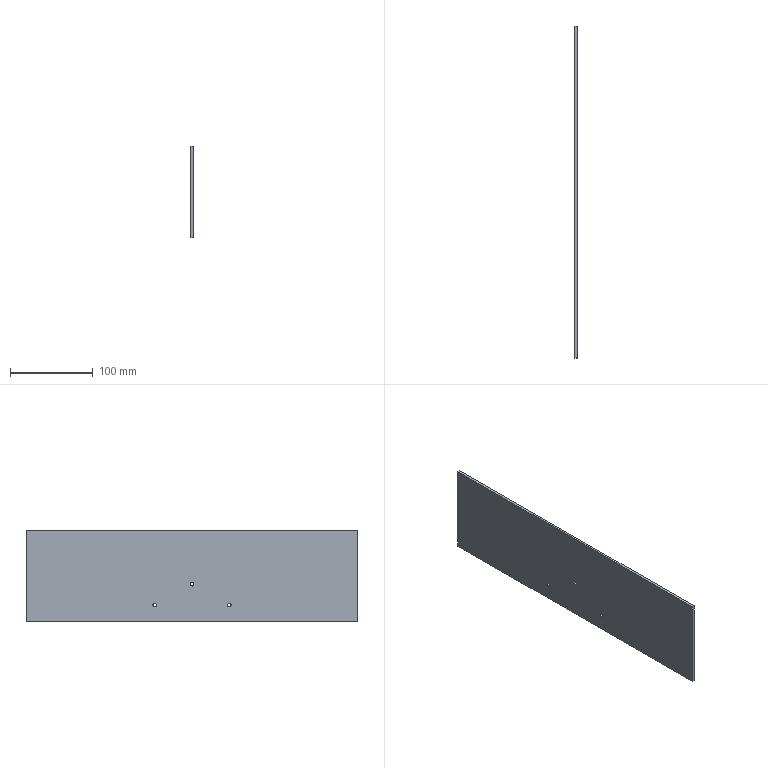Part | STEP file | HESS-408-70-15W-W-45-upper door right reinforcing plate | 1 solid | 12 faces | box 3 x 400 x 110 mm | volume 131875 mm3 | cylinder 6 | plane 6 | commonest cylinder face diameters 4.2 x6
STEP:
#1=CARTESIAN_POINT('',(0.,0.,0.));
#2=DIRECTION('',(0.,0.,1.));
#3=DIRECTION('',(1.,0.,0.));
#4=AXIS2_PLACEMENT_3D('',#1,#2,#3);
#5=CARTESIAN_POINT('',(-3.,-45.,-37.1));
#6=VERTEX_POINT('',#5);
#7=CARTESIAN_POINT('',(0.,-45.,-37.1));
#8=VERTEX_POINT('',#7);
#9=CARTESIAN_POINT('',(0.,-45.,-37.1));
#10=DIRECTION('',(1.,0.,0.));
#11=VECTOR('',#10,1.);
#12=LINE('',#9,#11);
#13=CARTESIAN_POINT('',(0.,-45.,-35.));
#14=DIRECTION('',(1.,0.,0.));
#15=DIRECTION('',(0.,0.,-1.));
#16=AXIS2_PLACEMENT_3D('',#13,#14,#15);
#17=CYLINDRICAL_SURFACE('',#16,2.1);
#18=CARTESIAN_POINT('',(6.283,0.));
#19=DIRECTION('',(0.,1.));
#20=VECTOR('',#19,1.);
#21=LINE('',#18,#20);
#22=(GEOMETRIC_REPRESENTATION_CONTEXT(2)PARAMETRIC_REPRESENTATION_CONTEXT()REPRESENTATION_CONTEXT('',''));
#23=DEFINITIONAL_REPRESENTATION('',(#21),#22);
#24=PCURVE('',#17,#23);
#25=CARTESIAN_POINT('',(0.,-45.,-35.));
#26=DIRECTION('',(1.,0.,0.));
#27=DIRECTION('',(0.,0.,-1.));
#28=AXIS2_PLACEMENT_3D('',#25,#26,#27);
#29=CYLINDRICAL_SURFACE('',#28,2.1);
#30=CARTESIAN_POINT('',(0.,0.));
#31=DIRECTION('',(0.,1.));
#32=VECTOR('',#31,1.);
#33=LINE('',#30,#32);
#34=(GEOMETRIC_REPRESENTATION_CONTEXT(2)PARAMETRIC_REPRESENTATION_CONTEXT()REPRESENTATION_CONTEXT('',''));
#35=DEFINITIONAL_REPRESENTATION('',(#33),#34);
#36=PCURVE('',#29,#35);
#37=SURFACE_CURVE('',#12,(#24,#36),.PCURVE_S1.);
#38=EDGE_CURVE('',#6,#8,#37,.T.);
#39=ORIENTED_EDGE('',*,*,#38,.T.);
#40=CARTESIAN_POINT('',(0.,-45.,-32.9));
#41=VERTEX_POINT('',#40);
#42=CARTESIAN_POINT('',(0.,-45.,-35.));
#43=DIRECTION('',(-1.,0.,0.));
#44=DIRECTION('',(0.,0.,-1.));
#45=AXIS2_PLACEMENT_3D('',#42,#43,#44);
#46=CIRCLE('',#45,2.1);
#47=CARTESIAN_POINT('',(6.283,0.));
#48=DIRECTION('',(-1.,0.));
#49=VECTOR('',#48,1.);
#50=LINE('',#47,#49);
#51=(GEOMETRIC_REPRESENTATION_CONTEXT(2)PARAMETRIC_REPRESENTATION_CONTEXT()REPRESENTATION_CONTEXT('',''));
#52=DEFINITIONAL_REPRESENTATION('',(#50),#51);
#53=PCURVE('',#17,#52);
#54=CARTESIAN_POINT('',(0.,0.,0.));
#55=DIRECTION('',(-1.,0.,0.));
#56=DIRECTION('',(0.,0.,1.));
#57=AXIS2_PLACEMENT_3D('',#54,#55,#56);
#58=PLANE('',#57);
#59=CARTESIAN_POINT('',(-35.,-45.));
#60=DIRECTION('',(-1.,0.));
#61=AXIS2_PLACEMENT_2D('',#59,#60);
#62=CIRCLE('',#61,2.1);
#63=(GEOMETRIC_REPRESENTATION_CONTEXT(2)PARAMETRIC_REPRESENTATION_CONTEXT()REPRESENTATION_CONTEXT('',''));
#64=DEFINITIONAL_REPRESENTATION('',(#62),#63);
#65=PCURVE('',#58,#64);
#66=SURFACE_CURVE('',#46,(#53,#65),.PCURVE_S1.);
#67=EDGE_CURVE('',#8,#41,#66,.T.);
#68=ORIENTED_EDGE('',*,*,#67,.T.);
#69=CARTESIAN_POINT('',(-3.,-45.,-32.9));
#70=VERTEX_POINT('',#69);
#71=CARTESIAN_POINT('',(0.,-45.,-32.9));
#72=DIRECTION('',(1.,0.,0.));
#73=VECTOR('',#72,1.);
#74=LINE('',#71,#73);
#75=CARTESIAN_POINT('',(3.142,0.));
#76=DIRECTION('',(0.,1.));
#77=VECTOR('',#76,1.);
#78=LINE('',#75,#77);
#79=(GEOMETRIC_REPRESENTATION_CONTEXT(2)PARAMETRIC_REPRESENTATION_CONTEXT()REPRESENTATION_CONTEXT('',''));
#80=DEFINITIONAL_REPRESENTATION('',(#78),#79);
#81=PCURVE('',#17,#80);
#82=CARTESIAN_POINT('',(3.142,0.));
#83=DIRECTION('',(0.,1.));
#84=VECTOR('',#83,1.);
#85=LINE('',#82,#84);
#86=(GEOMETRIC_REPRESENTATION_CONTEXT(2)PARAMETRIC_REPRESENTATION_CONTEXT()REPRESENTATION_CONTEXT('',''));
#87=DEFINITIONAL_REPRESENTATION('',(#85),#86);
#88=PCURVE('',#29,#87);
#89=SURFACE_CURVE('',#74,(#81,#88),.PCURVE_S1.);
#90=EDGE_CURVE('',#70,#41,#89,.T.);
#91=ORIENTED_EDGE('',*,*,#90,.F.);
#92=CARTESIAN_POINT('',(-3.,-45.,-35.));
#93=DIRECTION('',(1.,0.,0.));
#94=DIRECTION('',(0.,0.,-1.));
#95=AXIS2_PLACEMENT_3D('',#92,#93,#94);
#96=CIRCLE('',#95,2.1);
#97=CARTESIAN_POINT('',(0.,-3.));
#98=DIRECTION('',(1.,0.));
#99=VECTOR('',#98,1.);
#100=LINE('',#97,#99);
#101=(GEOMETRIC_REPRESENTATION_CONTEXT(2)PARAMETRIC_REPRESENTATION_CONTEXT()REPRESENTATION_CONTEXT('',''));
#102=DEFINITIONAL_REPRESENTATION('',(#100),#101);
#103=PCURVE('',#17,#102);
#104=CARTESIAN_POINT('',(-3.,0.,0.));
#105=DIRECTION('',(-1.,0.,0.));
#106=DIRECTION('',(0.,0.,1.));
#107=AXIS2_PLACEMENT_3D('',#104,#105,#106);
#108=PLANE('',#107);
#109=CARTESIAN_POINT('',(-37.1,-45.));
#110=CARTESIAN_POINT('',(-37.1,-41.363));
#111=CARTESIAN_POINT('',(-33.95,-43.181));
#112=CARTESIAN_POINT('',(-30.8,-45.));
#113=CARTESIAN_POINT('',(-33.95,-46.819));
#114=CARTESIAN_POINT('',(-37.1,-48.637));
#115=CARTESIAN_POINT('',(-37.1,-45.));
#116=(BOUNDED_CURVE()B_SPLINE_CURVE(2,(#109,#110,#111,#112,#113,#114,#115),.UNSPECIFIED.,.T.,.F.)B_SPLINE_CURVE_WITH_KNOTS((1,2,2,2,2,1),(-2.094,0.,2.094,4.189,6.283,8.378),.UNSPECIFIED.)CURVE()GEOMETRIC_REPRESENTATION_ITEM()RATIONAL_B_SPLINE_CURVE((1.,0.5,1.,0.5,1.,0.5,1.))REPRESENTATION_ITEM(''));
#117=(GEOMETRIC_REPRESENTATION_CONTEXT(2)PARAMETRIC_REPRESENTATION_CONTEXT()REPRESENTATION_CONTEXT('',''));
#118=DEFINITIONAL_REPRESENTATION('',(#116),#117);
#119=PCURVE('',#108,#118);
#120=SURFACE_CURVE('',#96,(#103,#119),.PCURVE_S1.);
#121=EDGE_CURVE('',#70,#6,#120,.T.);
#122=ORIENTED_EDGE('',*,*,#121,.T.);
#123=EDGE_LOOP('',(#39,#68,#91,#122));
#124=FACE_BOUND('',#123,.F.);
#125=ADVANCED_FACE('',(#124),#17,.F.);
#126=CARTESIAN_POINT('',(-3.,0.,-12.1));
#127=VERTEX_POINT('',#126);
#128=CARTESIAN_POINT('',(0.,0.,-12.1));
#129=VERTEX_POINT('',#128);
#130=CARTESIAN_POINT('',(0.,0.,-12.1));
#131=DIRECTION('',(1.,0.,0.));
#132=VECTOR('',#131,1.);
#133=LINE('',#130,#132);
#134=CARTESIAN_POINT('',(0.,0.,-10.));
#135=DIRECTION('',(1.,0.,0.));
#136=DIRECTION('',(0.,0.,-1.));
#137=AXIS2_PLACEMENT_3D('',#134,#135,#136);
#138=CYLINDRICAL_SURFACE('',#137,2.1);
#139=CARTESIAN_POINT('',(6.283,0.));
#140=DIRECTION('',(0.,1.));
#141=VECTOR('',#140,1.);
#142=LINE('',#139,#141);
#143=(GEOMETRIC_REPRESENTATION_CONTEXT(2)PARAMETRIC_REPRESENTATION_CONTEXT()REPRESENTATION_CONTEXT('',''));
#144=DEFINITIONAL_REPRESENTATION('',(#142),#143);
#145=PCURVE('',#138,#144);
#146=CARTESIAN_POINT('',(0.,0.,-10.));
#147=DIRECTION('',(1.,0.,0.));
#148=DIRECTION('',(0.,0.,-1.));
#149=AXIS2_PLACEMENT_3D('',#146,#147,#148);
#150=CYLINDRICAL_SURFACE('',#149,2.1);
#151=CARTESIAN_POINT('',(0.,0.));
#152=DIRECTION('',(0.,1.));
#153=VECTOR('',#152,1.);
#154=LINE('',#151,#153);
#155=(GEOMETRIC_REPRESENTATION_CONTEXT(2)PARAMETRIC_REPRESENTATION_CONTEXT()REPRESENTATION_CONTEXT('',''));
#156=DEFINITIONAL_REPRESENTATION('',(#154),#155);
#157=PCURVE('',#150,#156);
#158=SURFACE_CURVE('',#133,(#145,#157),.PCURVE_S1.);
#159=EDGE_CURVE('',#127,#129,#158,.T.);
#160=ORIENTED_EDGE('',*,*,#159,.T.);
#161=CARTESIAN_POINT('',(0.,0.,-7.9));
#162=VERTEX_POINT('',#161);
#163=CARTESIAN_POINT('',(0.,0.,-10.));
#164=DIRECTION('',(-1.,0.,0.));
#165=DIRECTION('',(0.,0.,-1.));
#166=AXIS2_PLACEMENT_3D('',#163,#164,#165);
#167=CIRCLE('',#166,2.1);
#168=CARTESIAN_POINT('',(6.283,0.));
#169=DIRECTION('',(-1.,0.));
#170=VECTOR('',#169,1.);
#171=LINE('',#168,#170);
#172=(GEOMETRIC_REPRESENTATION_CONTEXT(2)PARAMETRIC_REPRESENTATION_CONTEXT()REPRESENTATION_CONTEXT('',''));
#173=DEFINITIONAL_REPRESENTATION('',(#171),#172);
#174=PCURVE('',#138,#173);
#175=CARTESIAN_POINT('',(-10.,0.));
#176=DIRECTION('',(-1.,0.));
#177=AXIS2_PLACEMENT_2D('',#175,#176);
#178=CIRCLE('',#177,2.1);
#179=(GEOMETRIC_REPRESENTATION_CONTEXT(2)PARAMETRIC_REPRESENTATION_CONTEXT()REPRESENTATION_CONTEXT('',''));
#180=DEFINITIONAL_REPRESENTATION('',(#178),#179);
#181=PCURVE('',#58,#180);
#182=SURFACE_CURVE('',#167,(#174,#181),.PCURVE_S1.);
#183=EDGE_CURVE('',#129,#162,#182,.T.);
#184=ORIENTED_EDGE('',*,*,#183,.T.);
#185=CARTESIAN_POINT('',(-3.,0.,-7.9));
#186=VERTEX_POINT('',#185);
#187=CARTESIAN_POINT('',(0.,0.,-7.9));
#188=DIRECTION('',(1.,0.,0.));
#189=VECTOR('',#188,1.);
#190=LINE('',#187,#189);
#191=CARTESIAN_POINT('',(3.142,0.));
#192=DIRECTION('',(0.,1.));
#193=VECTOR('',#192,1.);
#194=LINE('',#191,#193);
#195=(GEOMETRIC_REPRESENTATION_CONTEXT(2)PARAMETRIC_REPRESENTATION_CONTEXT()REPRESENTATION_CONTEXT('',''));
#196=DEFINITIONAL_REPRESENTATION('',(#194),#195);
#197=PCURVE('',#138,#196);
#198=CARTESIAN_POINT('',(3.142,0.));
#199=DIRECTION('',(0.,1.));
#200=VECTOR('',#199,1.);
#201=LINE('',#198,#200);
#202=(GEOMETRIC_REPRESENTATION_CONTEXT(2)PARAMETRIC_REPRESENTATION_CONTEXT()REPRESENTATION_CONTEXT('',''));
#203=DEFINITIONAL_REPRESENTATION('',(#201),#202);
#204=PCURVE('',#150,#203);
#205=SURFACE_CURVE('',#190,(#197,#204),.PCURVE_S1.);
#206=EDGE_CURVE('',#186,#162,#205,.T.);
#207=ORIENTED_EDGE('',*,*,#206,.F.);
#208=CARTESIAN_POINT('',(-3.,0.,-10.));
#209=DIRECTION('',(1.,0.,0.));
#210=DIRECTION('',(0.,0.,-1.));
#211=AXIS2_PLACEMENT_3D('',#208,#209,#210);
#212=CIRCLE('',#211,2.1);
#213=CARTESIAN_POINT('',(0.,-3.));
#214=DIRECTION('',(1.,0.));
#215=VECTOR('',#214,1.);
#216=LINE('',#213,#215);
#217=(GEOMETRIC_REPRESENTATION_CONTEXT(2)PARAMETRIC_REPRESENTATION_CONTEXT()REPRESENTATION_CONTEXT('',''));
#218=DEFINITIONAL_REPRESENTATION('',(#216),#217);
#219=PCURVE('',#138,#218);
#220=CARTESIAN_POINT('',(-12.1,0.));
#221=CARTESIAN_POINT('',(-12.1,3.637));
#222=CARTESIAN_POINT('',(-8.95,1.819));
#223=CARTESIAN_POINT('',(-5.8,0.));
#224=CARTESIAN_POINT('',(-8.95,-1.819));
#225=CARTESIAN_POINT('',(-12.1,-3.637));
#226=CARTESIAN_POINT('',(-12.1,0.));
#227=(BOUNDED_CURVE()B_SPLINE_CURVE(2,(#220,#221,#222,#223,#224,#225,#226),.UNSPECIFIED.,.T.,.F.)B_SPLINE_CURVE_WITH_KNOTS((1,2,2,2,2,1),(-2.094,0.,2.094,4.189,6.283,8.378),.UNSPECIFIED.)CURVE()GEOMETRIC_REPRESENTATION_ITEM()RATIONAL_B_SPLINE_CURVE((1.,0.5,1.,0.5,1.,0.5,1.))REPRESENTATION_ITEM(''));
#228=(GEOMETRIC_REPRESENTATION_CONTEXT(2)PARAMETRIC_REPRESENTATION_CONTEXT()REPRESENTATION_CONTEXT('',''));
#229=DEFINITIONAL_REPRESENTATION('',(#227),#228);
#230=PCURVE('',#108,#229);
#231=SURFACE_CURVE('',#212,(#219,#230),.PCURVE_S1.);
#232=EDGE_CURVE('',#186,#127,#231,.T.);
#233=ORIENTED_EDGE('',*,*,#232,.T.);
#234=EDGE_LOOP('',(#160,#184,#207,#233));
#235=FACE_BOUND('',#234,.F.);
#236=ADVANCED_FACE('',(#235),#138,.F.);
#237=CARTESIAN_POINT('',(-3.,45.,-37.1));
#238=VERTEX_POINT('',#237);
#239=CARTESIAN_POINT('',(0.,45.,-37.1));
#240=VERTEX_POINT('',#239);
#241=CARTESIAN_POINT('',(0.,45.,-37.1));
#242=DIRECTION('',(1.,0.,0.));
#243=VECTOR('',#242,1.);
#244=LINE('',#241,#243);
#245=CARTESIAN_POINT('',(0.,45.,-35.));
#246=DIRECTION('',(1.,0.,0.));
#247=DIRECTION('',(0.,0.,-1.));
#248=AXIS2_PLACEMENT_3D('',#245,#246,#247);
#249=CYLINDRICAL_SURFACE('',#248,2.1);
#250=CARTESIAN_POINT('',(6.283,0.));
#251=DIRECTION('',(0.,1.));
#252=VECTOR('',#251,1.);
#253=LINE('',#250,#252);
#254=(GEOMETRIC_REPRESENTATION_CONTEXT(2)PARAMETRIC_REPRESENTATION_CONTEXT()REPRESENTATION_CONTEXT('',''));
#255=DEFINITIONAL_REPRESENTATION('',(#253),#254);
#256=PCURVE('',#249,#255);
#257=CARTESIAN_POINT('',(0.,45.,-35.));
#258=DIRECTION('',(1.,0.,0.));
#259=DIRECTION('',(0.,0.,-1.));
#260=AXIS2_PLACEMENT_3D('',#257,#258,#259);
#261=CYLINDRICAL_SURFACE('',#260,2.1);
#262=CARTESIAN_POINT('',(0.,0.));
#263=DIRECTION('',(0.,1.));
#264=VECTOR('',#263,1.);
#265=LINE('',#262,#264);
#266=(GEOMETRIC_REPRESENTATION_CONTEXT(2)PARAMETRIC_REPRESENTATION_CONTEXT()REPRESENTATION_CONTEXT('',''));
#267=DEFINITIONAL_REPRESENTATION('',(#265),#266);
#268=PCURVE('',#261,#267);
#269=SURFACE_CURVE('',#244,(#256,#268),.PCURVE_S1.);
#270=EDGE_CURVE('',#238,#240,#269,.T.);
#271=ORIENTED_EDGE('',*,*,#270,.T.);
#272=CARTESIAN_POINT('',(0.,45.,-32.9));
#273=VERTEX_POINT('',#272);
#274=CARTESIAN_POINT('',(0.,45.,-35.));
#275=DIRECTION('',(-1.,0.,0.));
#276=DIRECTION('',(0.,0.,-1.));
#277=AXIS2_PLACEMENT_3D('',#274,#275,#276);
#278=CIRCLE('',#277,2.1);
#279=CARTESIAN_POINT('',(6.283,0.));
#280=DIRECTION('',(-1.,0.));
#281=VECTOR('',#280,1.);
#282=LINE('',#279,#281);
#283=(GEOMETRIC_REPRESENTATION_CONTEXT(2)PARAMETRIC_REPRESENTATION_CONTEXT()REPRESENTATION_CONTEXT('',''));
#284=DEFINITIONAL_REPRESENTATION('',(#282),#283);
#285=PCURVE('',#249,#284);
#286=CARTESIAN_POINT('',(-35.,45.));
#287=DIRECTION('',(-1.,0.));
#288=AXIS2_PLACEMENT_2D('',#286,#287);
#289=CIRCLE('',#288,2.1);
#290=(GEOMETRIC_REPRESENTATION_CONTEXT(2)PARAMETRIC_REPRESENTATION_CONTEXT()REPRESENTATION_CONTEXT('',''));
#291=DEFINITIONAL_REPRESENTATION('',(#289),#290);
#292=PCURVE('',#58,#291);
#293=SURFACE_CURVE('',#278,(#285,#292),.PCURVE_S1.);
#294=EDGE_CURVE('',#240,#273,#293,.T.);
#295=ORIENTED_EDGE('',*,*,#294,.T.);
#296=CARTESIAN_POINT('',(-3.,45.,-32.9));
#297=VERTEX_POINT('',#296);
#298=CARTESIAN_POINT('',(0.,45.,-32.9));
#299=DIRECTION('',(1.,0.,0.));
#300=VECTOR('',#299,1.);
#301=LINE('',#298,#300);
#302=CARTESIAN_POINT('',(3.142,0.));
#303=DIRECTION('',(0.,1.));
#304=VECTOR('',#303,1.);
#305=LINE('',#302,#304);
#306=(GEOMETRIC_REPRESENTATION_CONTEXT(2)PARAMETRIC_REPRESENTATION_CONTEXT()REPRESENTATION_CONTEXT('',''));
#307=DEFINITIONAL_REPRESENTATION('',(#305),#306);
#308=PCURVE('',#249,#307);
#309=CARTESIAN_POINT('',(3.142,0.));
#310=DIRECTION('',(0.,1.));
#311=VECTOR('',#310,1.);
#312=LINE('',#309,#311);
#313=(GEOMETRIC_REPRESENTATION_CONTEXT(2)PARAMETRIC_REPRESENTATION_CONTEXT()REPRESENTATION_CONTEXT('',''));
#314=DEFINITIONAL_REPRESENTATION('',(#312),#313);
#315=PCURVE('',#261,#314);
#316=SURFACE_CURVE('',#301,(#308,#315),.PCURVE_S1.);
#317=EDGE_CURVE('',#297,#273,#316,.T.);
#318=ORIENTED_EDGE('',*,*,#317,.F.);
#319=CARTESIAN_POINT('',(-3.,45.,-35.));
#320=DIRECTION('',(1.,0.,0.));
#321=DIRECTION('',(0.,0.,-1.));
#322=AXIS2_PLACEMENT_3D('',#319,#320,#321);
#323=CIRCLE('',#322,2.1);
#324=CARTESIAN_POINT('',(0.,-3.));
#325=DIRECTION('',(1.,0.));
#326=VECTOR('',#325,1.);
#327=LINE('',#324,#326);
#328=(GEOMETRIC_REPRESENTATION_CONTEXT(2)PARAMETRIC_REPRESENTATION_CONTEXT()REPRESENTATION_CONTEXT('',''));
#329=DEFINITIONAL_REPRESENTATION('',(#327),#328);
#330=PCURVE('',#249,#329);
#331=CARTESIAN_POINT('',(-37.1,45.));
#332=CARTESIAN_POINT('',(-37.1,48.637));
#333=CARTESIAN_POINT('',(-33.95,46.819));
#334=CARTESIAN_POINT('',(-30.8,45.));
#335=CARTESIAN_POINT('',(-33.95,43.181));
#336=CARTESIAN_POINT('',(-37.1,41.363));
#337=CARTESIAN_POINT('',(-37.1,45.));
#338=(BOUNDED_CURVE()B_SPLINE_CURVE(2,(#331,#332,#333,#334,#335,#336,#337),.UNSPECIFIED.,.T.,.F.)B_SPLINE_CURVE_WITH_KNOTS((1,2,2,2,2,1),(-2.094,0.,2.094,4.189,6.283,8.378),.UNSPECIFIED.)CURVE()GEOMETRIC_REPRESENTATION_ITEM()RATIONAL_B_SPLINE_CURVE((1.,0.5,1.,0.5,1.,0.5,1.))REPRESENTATION_ITEM(''));
#339=(GEOMETRIC_REPRESENTATION_CONTEXT(2)PARAMETRIC_REPRESENTATION_CONTEXT()REPRESENTATION_CONTEXT('',''));
#340=DEFINITIONAL_REPRESENTATION('',(#338),#339);
#341=PCURVE('',#108,#340);
#342=SURFACE_CURVE('',#323,(#330,#341),.PCURVE_S1.);
#343=EDGE_CURVE('',#297,#238,#342,.T.);
#344=ORIENTED_EDGE('',*,*,#343,.T.);
#345=EDGE_LOOP('',(#271,#295,#318,#344));
#346=FACE_BOUND('',#345,.F.);
#347=ADVANCED_FACE('',(#346),#249,.F.);
#348=CARTESIAN_POINT('',(-3.,-200.,55.));
#349=VERTEX_POINT('',#348);
#350=CARTESIAN_POINT('',(-3.,200.,55.));
#351=VERTEX_POINT('',#350);
#352=CARTESIAN_POINT('',(-3.,0.,55.));
#353=DIRECTION('',(0.,1.,0.));
#354=VECTOR('',#353,1.);
#355=LINE('',#352,#354);
#356=CARTESIAN_POINT('',(55.,0.));
#357=DIRECTION('',(0.,1.));
#358=VECTOR('',#357,1.);
#359=LINE('',#356,#358);
#360=(GEOMETRIC_REPRESENTATION_CONTEXT(2)PARAMETRIC_REPRESENTATION_CONTEXT()REPRESENTATION_CONTEXT('',''));
#361=DEFINITIONAL_REPRESENTATION('',(#359),#360);
#362=PCURVE('',#108,#361);
#363=CARTESIAN_POINT('',(-3.,-200.,55.));
#364=DIRECTION('',(0.,0.,1.));
#365=DIRECTION('',(1.,0.,0.));
#366=AXIS2_PLACEMENT_3D('',#363,#364,#365);
#367=PLANE('',#366);
#368=CARTESIAN_POINT('',(0.,200.));
#369=DIRECTION('',(0.,1.));
#370=VECTOR('',#369,1.);
#371=LINE('',#368,#370);
#372=(GEOMETRIC_REPRESENTATION_CONTEXT(2)PARAMETRIC_REPRESENTATION_CONTEXT()REPRESENTATION_CONTEXT('',''));
#373=DEFINITIONAL_REPRESENTATION('',(#371),#372);
#374=PCURVE('',#367,#373);
#375=SURFACE_CURVE('',#355,(#362,#374),.PCURVE_S1.);
#376=EDGE_CURVE('',#349,#351,#375,.T.);
#377=ORIENTED_EDGE('',*,*,#376,.T.);
#378=CARTESIAN_POINT('',(-3.,200.,-55.));
#379=VERTEX_POINT('',#378);
#380=CARTESIAN_POINT('',(-3.,200.,0.));
#381=DIRECTION('',(0.,0.,-1.));
#382=VECTOR('',#381,1.);
#383=LINE('',#380,#382);
#384=CARTESIAN_POINT('',(0.,200.));
#385=DIRECTION('',(-1.,0.));
#386=VECTOR('',#385,1.);
#387=LINE('',#384,#386);
#388=(GEOMETRIC_REPRESENTATION_CONTEXT(2)PARAMETRIC_REPRESENTATION_CONTEXT()REPRESENTATION_CONTEXT('',''));
#389=DEFINITIONAL_REPRESENTATION('',(#387),#388);
#390=PCURVE('',#108,#389);
#391=CARTESIAN_POINT('',(-3.,200.,55.));
#392=DIRECTION('',(0.,1.,0.));
#393=DIRECTION('',(0.,0.,1.));
#394=AXIS2_PLACEMENT_3D('',#391,#392,#393);
#395=PLANE('',#394);
#396=CARTESIAN_POINT('',(-55.,0.));
#397=DIRECTION('',(-1.,0.));
#398=VECTOR('',#397,1.);
#399=LINE('',#396,#398);
#400=(GEOMETRIC_REPRESENTATION_CONTEXT(2)PARAMETRIC_REPRESENTATION_CONTEXT()REPRESENTATION_CONTEXT('',''));
#401=DEFINITIONAL_REPRESENTATION('',(#399),#400);
#402=PCURVE('',#395,#401);
#403=SURFACE_CURVE('',#383,(#390,#402),.PCURVE_S1.);
#404=EDGE_CURVE('',#351,#379,#403,.T.);
#405=ORIENTED_EDGE('',*,*,#404,.T.);
#406=CARTESIAN_POINT('',(-3.,-200.,-55.));
#407=VERTEX_POINT('',#406);
#408=CARTESIAN_POINT('',(-3.,0.,-55.));
#409=DIRECTION('',(0.,-1.,0.));
#410=VECTOR('',#409,1.);
#411=LINE('',#408,#410);
#412=CARTESIAN_POINT('',(-55.,0.));
#413=DIRECTION('',(0.,-1.));
#414=VECTOR('',#413,1.);
#415=LINE('',#412,#414);
#416=(GEOMETRIC_REPRESENTATION_CONTEXT(2)PARAMETRIC_REPRESENTATION_CONTEXT()REPRESENTATION_CONTEXT('',''));
#417=DEFINITIONAL_REPRESENTATION('',(#415),#416);
#418=PCURVE('',#108,#417);
#419=CARTESIAN_POINT('',(-3.,-200.,-55.));
#420=DIRECTION('',(0.,0.,-1.));
#421=DIRECTION('',(-1.,0.,0.));
#422=AXIS2_PLACEMENT_3D('',#419,#420,#421);
#423=PLANE('',#422);
#424=CARTESIAN_POINT('',(0.,200.));
#425=DIRECTION('',(0.,-1.));
#426=VECTOR('',#425,1.);
#427=LINE('',#424,#426);
#428=(GEOMETRIC_REPRESENTATION_CONTEXT(2)PARAMETRIC_REPRESENTATION_CONTEXT()REPRESENTATION_CONTEXT('',''));
#429=DEFINITIONAL_REPRESENTATION('',(#427),#428);
#430=PCURVE('',#423,#429);
#431=SURFACE_CURVE('',#411,(#418,#430),.PCURVE_S1.);
#432=EDGE_CURVE('',#379,#407,#431,.T.);
#433=ORIENTED_EDGE('',*,*,#432,.T.);
#434=CARTESIAN_POINT('',(-3.,-200.,0.));
#435=DIRECTION('',(0.,0.,1.));
#436=VECTOR('',#435,1.);
#437=LINE('',#434,#436);
#438=CARTESIAN_POINT('',(0.,-200.));
#439=DIRECTION('',(1.,0.));
#440=VECTOR('',#439,1.);
#441=LINE('',#438,#440);
#442=(GEOMETRIC_REPRESENTATION_CONTEXT(2)PARAMETRIC_REPRESENTATION_CONTEXT()REPRESENTATION_CONTEXT('',''));
#443=DEFINITIONAL_REPRESENTATION('',(#441),#442);
#444=PCURVE('',#108,#443);
#445=CARTESIAN_POINT('',(-3.,-200.,55.));
#446=DIRECTION('',(0.,-1.,0.));
#447=DIRECTION('',(0.,0.,-1.));
#448=AXIS2_PLACEMENT_3D('',#445,#446,#447);
#449=PLANE('',#448);
#450=CARTESIAN_POINT('',(55.,0.));
#451=DIRECTION('',(-1.,0.));
#452=VECTOR('',#451,1.);
#453=LINE('',#450,#452);
#454=(GEOMETRIC_REPRESENTATION_CONTEXT(2)PARAMETRIC_REPRESENTATION_CONTEXT()REPRESENTATION_CONTEXT('',''));
#455=DEFINITIONAL_REPRESENTATION('',(#453),#454);
#456=PCURVE('',#449,#455);
#457=SURFACE_CURVE('',#437,(#444,#456),.PCURVE_S1.);
#458=EDGE_CURVE('',#407,#349,#457,.T.);
#459=ORIENTED_EDGE('',*,*,#458,.T.);
#460=EDGE_LOOP('',(#377,#405,#433,#459));
#461=FACE_BOUND('',#460,.T.);
#462=CARTESIAN_POINT('',(-3.,-45.,-35.));
#463=DIRECTION('',(1.,0.,0.));
#464=DIRECTION('',(0.,0.,-1.));
#465=AXIS2_PLACEMENT_3D('',#462,#463,#464);
#466=CIRCLE('',#465,2.1);
#467=CARTESIAN_POINT('',(-37.1,-45.));
#468=CARTESIAN_POINT('',(-37.1,-41.363));
#469=CARTESIAN_POINT('',(-33.95,-43.181));
#470=CARTESIAN_POINT('',(-30.8,-45.));
#471=CARTESIAN_POINT('',(-33.95,-46.819));
#472=CARTESIAN_POINT('',(-37.1,-48.637));
#473=CARTESIAN_POINT('',(-37.1,-45.));
#474=(BOUNDED_CURVE()B_SPLINE_CURVE(2,(#467,#468,#469,#470,#471,#472,#473),.UNSPECIFIED.,.T.,.F.)B_SPLINE_CURVE_WITH_KNOTS((1,2,2,2,2,1),(-2.094,0.,2.094,4.189,6.283,8.378),.UNSPECIFIED.)CURVE()GEOMETRIC_REPRESENTATION_ITEM()RATIONAL_B_SPLINE_CURVE((1.,0.5,1.,0.5,1.,0.5,1.))REPRESENTATION_ITEM(''));
#475=(GEOMETRIC_REPRESENTATION_CONTEXT(2)PARAMETRIC_REPRESENTATION_CONTEXT()REPRESENTATION_CONTEXT('',''));
#476=DEFINITIONAL_REPRESENTATION('',(#474),#475);
#477=PCURVE('',#108,#476);
#478=CARTESIAN_POINT('',(0.,-3.));
#479=DIRECTION('',(1.,0.));
#480=VECTOR('',#479,1.);
#481=LINE('',#478,#480);
#482=(GEOMETRIC_REPRESENTATION_CONTEXT(2)PARAMETRIC_REPRESENTATION_CONTEXT()REPRESENTATION_CONTEXT('',''));
#483=DEFINITIONAL_REPRESENTATION('',(#481),#482);
#484=PCURVE('',#29,#483);
#485=SURFACE_CURVE('',#466,(#477,#484),.PCURVE_S1.);
#486=EDGE_CURVE('',#6,#70,#485,.T.);
#487=ORIENTED_EDGE('',*,*,#486,.T.);
#488=ORIENTED_EDGE('',*,*,#121,.T.);
#489=EDGE_LOOP('',(#487,#488));
#490=FACE_BOUND('',#489,.T.);
#491=CARTESIAN_POINT('',(-3.,0.,-10.));
#492=DIRECTION('',(1.,0.,0.));
#493=DIRECTION('',(0.,0.,-1.));
#494=AXIS2_PLACEMENT_3D('',#491,#492,#493);
#495=CIRCLE('',#494,2.1);
#496=CARTESIAN_POINT('',(-12.1,0.));
#497=CARTESIAN_POINT('',(-12.1,3.637));
#498=CARTESIAN_POINT('',(-8.95,1.819));
#499=CARTESIAN_POINT('',(-5.8,0.));
#500=CARTESIAN_POINT('',(-8.95,-1.819));
#501=CARTESIAN_POINT('',(-12.1,-3.637));
#502=CARTESIAN_POINT('',(-12.1,0.));
#503=(BOUNDED_CURVE()B_SPLINE_CURVE(2,(#496,#497,#498,#499,#500,#501,#502),.UNSPECIFIED.,.T.,.F.)B_SPLINE_CURVE_WITH_KNOTS((1,2,2,2,2,1),(-2.094,0.,2.094,4.189,6.283,8.378),.UNSPECIFIED.)CURVE()GEOMETRIC_REPRESENTATION_ITEM()RATIONAL_B_SPLINE_CURVE((1.,0.5,1.,0.5,1.,0.5,1.))REPRESENTATION_ITEM(''));
#504=(GEOMETRIC_REPRESENTATION_CONTEXT(2)PARAMETRIC_REPRESENTATION_CONTEXT()REPRESENTATION_CONTEXT('',''));
#505=DEFINITIONAL_REPRESENTATION('',(#503),#504);
#506=PCURVE('',#108,#505);
#507=CARTESIAN_POINT('',(0.,-3.));
#508=DIRECTION('',(1.,0.));
#509=VECTOR('',#508,1.);
#510=LINE('',#507,#509);
#511=(GEOMETRIC_REPRESENTATION_CONTEXT(2)PARAMETRIC_REPRESENTATION_CONTEXT()REPRESENTATION_CONTEXT('',''));
#512=DEFINITIONAL_REPRESENTATION('',(#510),#511);
#513=PCURVE('',#150,#512);
#514=SURFACE_CURVE('',#495,(#506,#513),.PCURVE_S1.);
#515=EDGE_CURVE('',#127,#186,#514,.T.);
#516=ORIENTED_EDGE('',*,*,#515,.T.);
#517=ORIENTED_EDGE('',*,*,#232,.T.);
#518=EDGE_LOOP('',(#516,#517));
#519=FACE_BOUND('',#518,.T.);
#520=CARTESIAN_POINT('',(-3.,45.,-35.));
#521=DIRECTION('',(1.,0.,0.));
#522=DIRECTION('',(0.,0.,-1.));
#523=AXIS2_PLACEMENT_3D('',#520,#521,#522);
#524=CIRCLE('',#523,2.1);
#525=CARTESIAN_POINT('',(-37.1,45.));
#526=CARTESIAN_POINT('',(-37.1,48.637));
#527=CARTESIAN_POINT('',(-33.95,46.819));
#528=CARTESIAN_POINT('',(-30.8,45.));
#529=CARTESIAN_POINT('',(-33.95,43.181));
#530=CARTESIAN_POINT('',(-37.1,41.363));
#531=CARTESIAN_POINT('',(-37.1,45.));
#532=(BOUNDED_CURVE()B_SPLINE_CURVE(2,(#525,#526,#527,#528,#529,#530,#531),.UNSPECIFIED.,.T.,.F.)B_SPLINE_CURVE_WITH_KNOTS((1,2,2,2,2,1),(-2.094,0.,2.094,4.189,6.283,8.378),.UNSPECIFIED.)CURVE()GEOMETRIC_REPRESENTATION_ITEM()RATIONAL_B_SPLINE_CURVE((1.,0.5,1.,0.5,1.,0.5,1.))REPRESENTATION_ITEM(''));
#533=(GEOMETRIC_REPRESENTATION_CONTEXT(2)PARAMETRIC_REPRESENTATION_CONTEXT()REPRESENTATION_CONTEXT('',''));
#534=DEFINITIONAL_REPRESENTATION('',(#532),#533);
#535=PCURVE('',#108,#534);
#536=CARTESIAN_POINT('',(0.,-3.));
#537=DIRECTION('',(1.,0.));
#538=VECTOR('',#537,1.);
#539=LINE('',#536,#538);
#540=(GEOMETRIC_REPRESENTATION_CONTEXT(2)PARAMETRIC_REPRESENTATION_CONTEXT()REPRESENTATION_CONTEXT('',''));
#541=DEFINITIONAL_REPRESENTATION('',(#539),#540);
#542=PCURVE('',#261,#541);
#543=SURFACE_CURVE('',#524,(#535,#542),.PCURVE_S1.);
#544=EDGE_CURVE('',#238,#297,#543,.T.);
#545=ORIENTED_EDGE('',*,*,#544,.T.);
#546=ORIENTED_EDGE('',*,*,#343,.T.);
#547=EDGE_LOOP('',(#545,#546));
#548=FACE_BOUND('',#547,.T.);
#549=ADVANCED_FACE('',(#461,#490,#519,#548),#108,.T.);
#550=ORIENTED_EDGE('',*,*,#404,.F.);
#551=CARTESIAN_POINT('',(0.,200.,55.));
#552=VERTEX_POINT('',#551);
#553=CARTESIAN_POINT('',(-3.,200.,55.));
#554=DIRECTION('',(1.,0.,0.));
#555=VECTOR('',#554,1.);
#556=LINE('',#553,#555);
#557=CARTESIAN_POINT('',(0.,0.));
#558=DIRECTION('',(0.,1.));
#559=VECTOR('',#558,1.);
#560=LINE('',#557,#559);
#561=(GEOMETRIC_REPRESENTATION_CONTEXT(2)PARAMETRIC_REPRESENTATION_CONTEXT()REPRESENTATION_CONTEXT('',''));
#562=DEFINITIONAL_REPRESENTATION('',(#560),#561);
#563=PCURVE('',#395,#562);
#564=CARTESIAN_POINT('',(0.,400.));
#565=DIRECTION('',(1.,0.));
#566=VECTOR('',#565,1.);
#567=LINE('',#564,#566);
#568=(GEOMETRIC_REPRESENTATION_CONTEXT(2)PARAMETRIC_REPRESENTATION_CONTEXT()REPRESENTATION_CONTEXT('',''));
#569=DEFINITIONAL_REPRESENTATION('',(#567),#568);
#570=PCURVE('',#367,#569);
#571=SURFACE_CURVE('',#556,(#563,#570),.PCURVE_S1.);
#572=EDGE_CURVE('',#351,#552,#571,.T.);
#573=ORIENTED_EDGE('',*,*,#572,.T.);
#574=CARTESIAN_POINT('',(0.,200.,-55.));
#575=VERTEX_POINT('',#574);
#576=CARTESIAN_POINT('',(0.,200.,55.));
#577=DIRECTION('',(0.,0.,-1.));
#578=VECTOR('',#577,1.);
#579=LINE('',#576,#578);
#580=CARTESIAN_POINT('',(0.,3.));
#581=DIRECTION('',(-1.,0.));
#582=VECTOR('',#581,1.);
#583=LINE('',#580,#582);
#584=(GEOMETRIC_REPRESENTATION_CONTEXT(2)PARAMETRIC_REPRESENTATION_CONTEXT()REPRESENTATION_CONTEXT('',''));
#585=DEFINITIONAL_REPRESENTATION('',(#583),#584);
#586=PCURVE('',#395,#585);
#587=CARTESIAN_POINT('',(55.,200.));
#588=DIRECTION('',(-1.,0.));
#589=VECTOR('',#588,1.);
#590=LINE('',#587,#589);
#591=(GEOMETRIC_REPRESENTATION_CONTEXT(2)PARAMETRIC_REPRESENTATION_CONTEXT()REPRESENTATION_CONTEXT('',''));
#592=DEFINITIONAL_REPRESENTATION('',(#590),#591);
#593=PCURVE('',#58,#592);
#594=SURFACE_CURVE('',#579,(#586,#593),.PCURVE_S1.);
#595=EDGE_CURVE('',#552,#575,#594,.T.);
#596=ORIENTED_EDGE('',*,*,#595,.T.);
#597=CARTESIAN_POINT('',(-3.,200.,-55.));
#598=DIRECTION('',(-1.,0.,0.));
#599=VECTOR('',#598,1.);
#600=LINE('',#597,#599);
#601=CARTESIAN_POINT('',(-110.,0.));
#602=DIRECTION('',(0.,-1.));
#603=VECTOR('',#602,1.);
#604=LINE('',#601,#603);
#605=(GEOMETRIC_REPRESENTATION_CONTEXT(2)PARAMETRIC_REPRESENTATION_CONTEXT()REPRESENTATION_CONTEXT('',''));
#606=DEFINITIONAL_REPRESENTATION('',(#604),#605);
#607=PCURVE('',#395,#606);
#608=CARTESIAN_POINT('',(0.,400.));
#609=DIRECTION('',(1.,0.));
#610=VECTOR('',#609,1.);
#611=LINE('',#608,#610);
#612=(GEOMETRIC_REPRESENTATION_CONTEXT(2)PARAMETRIC_REPRESENTATION_CONTEXT()REPRESENTATION_CONTEXT('',''));
#613=DEFINITIONAL_REPRESENTATION('',(#611),#612);
#614=PCURVE('',#423,#613);
#615=SURFACE_CURVE('',#600,(#607,#614),.PCURVE_S1.);
#616=EDGE_CURVE('',#575,#379,#615,.T.);
#617=ORIENTED_EDGE('',*,*,#616,.T.);
#618=EDGE_LOOP('',(#550,#573,#596,#617));
#619=FACE_BOUND('',#618,.T.);
#620=ADVANCED_FACE('',(#619),#395,.T.);
#621=ORIENTED_EDGE('',*,*,#376,.F.);
#622=CARTESIAN_POINT('',(0.,-200.,55.));
#623=VERTEX_POINT('',#622);
#624=CARTESIAN_POINT('',(-3.,-200.,55.));
#625=DIRECTION('',(1.,0.,0.));
#626=VECTOR('',#625,1.);
#627=LINE('',#624,#626);
#628=CARTESIAN_POINT('',(0.,0.));
#629=DIRECTION('',(1.,0.));
#630=VECTOR('',#629,1.);
#631=LINE('',#628,#630);
#632=(GEOMETRIC_REPRESENTATION_CONTEXT(2)PARAMETRIC_REPRESENTATION_CONTEXT()REPRESENTATION_CONTEXT('',''));
#633=DEFINITIONAL_REPRESENTATION('',(#631),#632);
#634=PCURVE('',#367,#633);
#635=CARTESIAN_POINT('',(0.,0.));
#636=DIRECTION('',(0.,1.));
#637=VECTOR('',#636,1.);
#638=LINE('',#635,#637);
#639=(GEOMETRIC_REPRESENTATION_CONTEXT(2)PARAMETRIC_REPRESENTATION_CONTEXT()REPRESENTATION_CONTEXT('',''));
#640=DEFINITIONAL_REPRESENTATION('',(#638),#639);
#641=PCURVE('',#449,#640);
#642=SURFACE_CURVE('',#627,(#634,#641),.PCURVE_S1.);
#643=EDGE_CURVE('',#349,#623,#642,.T.);
#644=ORIENTED_EDGE('',*,*,#643,.T.);
#645=CARTESIAN_POINT('',(0.,-200.,55.));
#646=DIRECTION('',(0.,1.,0.));
#647=VECTOR('',#646,1.);
#648=LINE('',#645,#647);
#649=CARTESIAN_POINT('',(3.,0.));
#650=DIRECTION('',(0.,1.));
#651=VECTOR('',#650,1.);
#652=LINE('',#649,#651);
#653=(GEOMETRIC_REPRESENTATION_CONTEXT(2)PARAMETRIC_REPRESENTATION_CONTEXT()REPRESENTATION_CONTEXT('',''));
#654=DEFINITIONAL_REPRESENTATION('',(#652),#653);
#655=PCURVE('',#367,#654);
#656=CARTESIAN_POINT('',(55.,-200.));
#657=DIRECTION('',(0.,1.));
#658=VECTOR('',#657,1.);
#659=LINE('',#656,#658);
#660=(GEOMETRIC_REPRESENTATION_CONTEXT(2)PARAMETRIC_REPRESENTATION_CONTEXT()REPRESENTATION_CONTEXT('',''));
#661=DEFINITIONAL_REPRESENTATION('',(#659),#660);
#662=PCURVE('',#58,#661);
#663=SURFACE_CURVE('',#648,(#655,#662),.PCURVE_S1.);
#664=EDGE_CURVE('',#623,#552,#663,.T.);
#665=ORIENTED_EDGE('',*,*,#664,.T.);
#666=ORIENTED_EDGE('',*,*,#572,.F.);
#667=EDGE_LOOP('',(#621,#644,#665,#666));
#668=FACE_BOUND('',#667,.T.);
#669=ADVANCED_FACE('',(#668),#367,.T.);
#670=ORIENTED_EDGE('',*,*,#458,.F.);
#671=CARTESIAN_POINT('',(0.,-200.,-55.));
#672=VERTEX_POINT('',#671);
#673=CARTESIAN_POINT('',(-3.,-200.,-55.));
#674=DIRECTION('',(1.,0.,0.));
#675=VECTOR('',#674,1.);
#676=LINE('',#673,#675);
#677=CARTESIAN_POINT('',(110.,0.));
#678=DIRECTION('',(0.,1.));
#679=VECTOR('',#678,1.);
#680=LINE('',#677,#679);
#681=(GEOMETRIC_REPRESENTATION_CONTEXT(2)PARAMETRIC_REPRESENTATION_CONTEXT()REPRESENTATION_CONTEXT('',''));
#682=DEFINITIONAL_REPRESENTATION('',(#680),#681);
#683=PCURVE('',#449,#682);
#684=CARTESIAN_POINT('',(0.,0.));
#685=DIRECTION('',(-1.,0.));
#686=VECTOR('',#685,1.);
#687=LINE('',#684,#686);
#688=(GEOMETRIC_REPRESENTATION_CONTEXT(2)PARAMETRIC_REPRESENTATION_CONTEXT()REPRESENTATION_CONTEXT('',''));
#689=DEFINITIONAL_REPRESENTATION('',(#687),#688);
#690=PCURVE('',#423,#689);
#691=SURFACE_CURVE('',#676,(#683,#690),.PCURVE_S1.);
#692=EDGE_CURVE('',#407,#672,#691,.T.);
#693=ORIENTED_EDGE('',*,*,#692,.T.);
#694=CARTESIAN_POINT('',(0.,-200.,55.));
#695=DIRECTION('',(0.,0.,1.));
#696=VECTOR('',#695,1.);
#697=LINE('',#694,#696);
#698=CARTESIAN_POINT('',(0.,3.));
#699=DIRECTION('',(-1.,0.));
#700=VECTOR('',#699,1.);
#701=LINE('',#698,#700);
#702=(GEOMETRIC_REPRESENTATION_CONTEXT(2)PARAMETRIC_REPRESENTATION_CONTEXT()REPRESENTATION_CONTEXT('',''));
#703=DEFINITIONAL_REPRESENTATION('',(#701),#702);
#704=PCURVE('',#449,#703);
#705=CARTESIAN_POINT('',(55.,-200.));
#706=DIRECTION('',(1.,0.));
#707=VECTOR('',#706,1.);
#708=LINE('',#705,#707);
#709=(GEOMETRIC_REPRESENTATION_CONTEXT(2)PARAMETRIC_REPRESENTATION_CONTEXT()REPRESENTATION_CONTEXT('',''));
#710=DEFINITIONAL_REPRESENTATION('',(#708),#709);
#711=PCURVE('',#58,#710);
#712=SURFACE_CURVE('',#697,(#704,#711),.PCURVE_S1.);
#713=EDGE_CURVE('',#672,#623,#712,.T.);
#714=ORIENTED_EDGE('',*,*,#713,.T.);
#715=ORIENTED_EDGE('',*,*,#643,.F.);
#716=EDGE_LOOP('',(#670,#693,#714,#715));
#717=FACE_BOUND('',#716,.T.);
#718=ADVANCED_FACE('',(#717),#449,.T.);
#719=ORIENTED_EDGE('',*,*,#432,.F.);
#720=ORIENTED_EDGE('',*,*,#616,.F.);
#721=CARTESIAN_POINT('',(0.,-200.,-55.));
#722=DIRECTION('',(0.,-1.,0.));
#723=VECTOR('',#722,1.);
#724=LINE('',#721,#723);
#725=CARTESIAN_POINT('',(-3.,0.));
#726=DIRECTION('',(0.,-1.));
#727=VECTOR('',#726,1.);
#728=LINE('',#725,#727);
#729=(GEOMETRIC_REPRESENTATION_CONTEXT(2)PARAMETRIC_REPRESENTATION_CONTEXT()REPRESENTATION_CONTEXT('',''));
#730=DEFINITIONAL_REPRESENTATION('',(#728),#729);
#731=PCURVE('',#423,#730);
#732=CARTESIAN_POINT('',(-55.,-200.));
#733=DIRECTION('',(0.,-1.));
#734=VECTOR('',#733,1.);
#735=LINE('',#732,#734);
#736=(GEOMETRIC_REPRESENTATION_CONTEXT(2)PARAMETRIC_REPRESENTATION_CONTEXT()REPRESENTATION_CONTEXT('',''));
#737=DEFINITIONAL_REPRESENTATION('',(#735),#736);
#738=PCURVE('',#58,#737);
#739=SURFACE_CURVE('',#724,(#731,#738),.PCURVE_S1.);
#740=EDGE_CURVE('',#575,#672,#739,.T.);
#741=ORIENTED_EDGE('',*,*,#740,.T.);
#742=ORIENTED_EDGE('',*,*,#692,.F.);
#743=EDGE_LOOP('',(#719,#720,#741,#742));
#744=FACE_BOUND('',#743,.T.);
#745=ADVANCED_FACE('',(#744),#423,.T.);
#746=CARTESIAN_POINT('',(0.,-45.,-35.));
#747=DIRECTION('',(-1.,0.,0.));
#748=DIRECTION('',(0.,0.,-1.));
#749=AXIS2_PLACEMENT_3D('',#746,#747,#748);
#750=CIRCLE('',#749,2.1);
#751=CARTESIAN_POINT('',(6.283,0.));
#752=DIRECTION('',(-1.,0.));
#753=VECTOR('',#752,1.);
#754=LINE('',#751,#753);
#755=(GEOMETRIC_REPRESENTATION_CONTEXT(2)PARAMETRIC_REPRESENTATION_CONTEXT()REPRESENTATION_CONTEXT('',''));
#756=DEFINITIONAL_REPRESENTATION('',(#754),#755);
#757=PCURVE('',#29,#756);
#758=CARTESIAN_POINT('',(-35.,-45.));
#759=DIRECTION('',(-1.,0.));
#760=AXIS2_PLACEMENT_2D('',#758,#759);
#761=CIRCLE('',#760,2.1);
#762=(GEOMETRIC_REPRESENTATION_CONTEXT(2)PARAMETRIC_REPRESENTATION_CONTEXT()REPRESENTATION_CONTEXT('',''));
#763=DEFINITIONAL_REPRESENTATION('',(#761),#762);
#764=PCURVE('',#58,#763);
#765=SURFACE_CURVE('',#750,(#757,#764),.PCURVE_S1.);
#766=EDGE_CURVE('',#41,#8,#765,.T.);
#767=ORIENTED_EDGE('',*,*,#766,.T.);
#768=ORIENTED_EDGE('',*,*,#38,.F.);
#769=ORIENTED_EDGE('',*,*,#486,.T.);
#770=ORIENTED_EDGE('',*,*,#90,.T.);
#771=EDGE_LOOP('',(#767,#768,#769,#770));
#772=FACE_BOUND('',#771,.F.);
#773=ADVANCED_FACE('',(#772),#29,.F.);
#774=CARTESIAN_POINT('',(0.,0.,-10.));
#775=DIRECTION('',(-1.,0.,0.));
#776=DIRECTION('',(0.,0.,-1.));
#777=AXIS2_PLACEMENT_3D('',#774,#775,#776);
#778=CIRCLE('',#777,2.1);
#779=CARTESIAN_POINT('',(6.283,0.));
#780=DIRECTION('',(-1.,0.));
#781=VECTOR('',#780,1.);
#782=LINE('',#779,#781);
#783=(GEOMETRIC_REPRESENTATION_CONTEXT(2)PARAMETRIC_REPRESENTATION_CONTEXT()REPRESENTATION_CONTEXT('',''));
#784=DEFINITIONAL_REPRESENTATION('',(#782),#783);
#785=PCURVE('',#150,#784);
#786=CARTESIAN_POINT('',(-10.,0.));
#787=DIRECTION('',(-1.,0.));
#788=AXIS2_PLACEMENT_2D('',#786,#787);
#789=CIRCLE('',#788,2.1);
#790=(GEOMETRIC_REPRESENTATION_CONTEXT(2)PARAMETRIC_REPRESENTATION_CONTEXT()REPRESENTATION_CONTEXT('',''));
#791=DEFINITIONAL_REPRESENTATION('',(#789),#790);
#792=PCURVE('',#58,#791);
#793=SURFACE_CURVE('',#778,(#785,#792),.PCURVE_S1.);
#794=EDGE_CURVE('',#162,#129,#793,.T.);
#795=ORIENTED_EDGE('',*,*,#794,.T.);
#796=ORIENTED_EDGE('',*,*,#159,.F.);
#797=ORIENTED_EDGE('',*,*,#515,.T.);
#798=ORIENTED_EDGE('',*,*,#206,.T.);
#799=EDGE_LOOP('',(#795,#796,#797,#798));
#800=FACE_BOUND('',#799,.F.);
#801=ADVANCED_FACE('',(#800),#150,.F.);
#802=CARTESIAN_POINT('',(0.,45.,-35.));
#803=DIRECTION('',(-1.,0.,0.));
#804=DIRECTION('',(0.,0.,-1.));
#805=AXIS2_PLACEMENT_3D('',#802,#803,#804);
#806=CIRCLE('',#805,2.1);
#807=CARTESIAN_POINT('',(6.283,0.));
#808=DIRECTION('',(-1.,0.));
#809=VECTOR('',#808,1.);
#810=LINE('',#807,#809);
#811=(GEOMETRIC_REPRESENTATION_CONTEXT(2)PARAMETRIC_REPRESENTATION_CONTEXT()REPRESENTATION_CONTEXT('',''));
#812=DEFINITIONAL_REPRESENTATION('',(#810),#811);
#813=PCURVE('',#261,#812);
#814=CARTESIAN_POINT('',(-35.,45.));
#815=DIRECTION('',(-1.,0.));
#816=AXIS2_PLACEMENT_2D('',#814,#815);
#817=CIRCLE('',#816,2.1);
#818=(GEOMETRIC_REPRESENTATION_CONTEXT(2)PARAMETRIC_REPRESENTATION_CONTEXT()REPRESENTATION_CONTEXT('',''));
#819=DEFINITIONAL_REPRESENTATION('',(#817),#818);
#820=PCURVE('',#58,#819);
#821=SURFACE_CURVE('',#806,(#813,#820),.PCURVE_S1.);
#822=EDGE_CURVE('',#273,#240,#821,.T.);
#823=ORIENTED_EDGE('',*,*,#822,.T.);
#824=ORIENTED_EDGE('',*,*,#270,.F.);
#825=ORIENTED_EDGE('',*,*,#544,.T.);
#826=ORIENTED_EDGE('',*,*,#317,.T.);
#827=EDGE_LOOP('',(#823,#824,#825,#826));
#828=FACE_BOUND('',#827,.F.);
#829=ADVANCED_FACE('',(#828),#261,.F.);
#830=ORIENTED_EDGE('',*,*,#183,.T.);
#831=ORIENTED_EDGE('',*,*,#794,.T.);
#832=EDGE_LOOP('',(#830,#831));
#833=FACE_BOUND('',#832,.T.);
#834=ORIENTED_EDGE('',*,*,#595,.F.);
#835=ORIENTED_EDGE('',*,*,#664,.F.);
#836=ORIENTED_EDGE('',*,*,#713,.F.);
#837=ORIENTED_EDGE('',*,*,#740,.F.);
#838=EDGE_LOOP('',(#834,#835,#836,#837));
#839=FACE_BOUND('',#838,.T.);
#840=ORIENTED_EDGE('',*,*,#67,.T.);
#841=ORIENTED_EDGE('',*,*,#766,.T.);
#842=EDGE_LOOP('',(#840,#841));
#843=FACE_BOUND('',#842,.T.);
#844=ORIENTED_EDGE('',*,*,#294,.T.);
#845=ORIENTED_EDGE('',*,*,#822,.T.);
#846=EDGE_LOOP('',(#844,#845));
#847=FACE_BOUND('',#846,.T.);
#848=ADVANCED_FACE('',(#833,#839,#843,#847),#58,.F.);
#849=CLOSED_SHELL('',(#125,#236,#347,#549,#620,#669,#718,#745,#773,#801,#829,#848));
#850=MANIFOLD_SOLID_BREP('',#849);
#851=(LENGTH_UNIT()NAMED_UNIT(*)SI_UNIT(.MILLI.,.METRE.));
#852=UNCERTAINTY_MEASURE_WITH_UNIT(LENGTH_MEASURE(0.0000001),#851,'','');
#853=(NAMED_UNIT(*)PLANE_ANGLE_UNIT()SI_UNIT($,.RADIAN.));
#854=(NAMED_UNIT(*)SI_UNIT($,.STERADIAN.)SOLID_ANGLE_UNIT());
#855=(GEOMETRIC_REPRESENTATION_CONTEXT(3)GLOBAL_UNCERTAINTY_ASSIGNED_CONTEXT((#852))GLOBAL_UNIT_ASSIGNED_CONTEXT((#851,#853,#854))REPRESENTATION_CONTEXT('',''));
#856=ADVANCED_BREP_SHAPE_REPRESENTATION('',(#4,#850),#855);